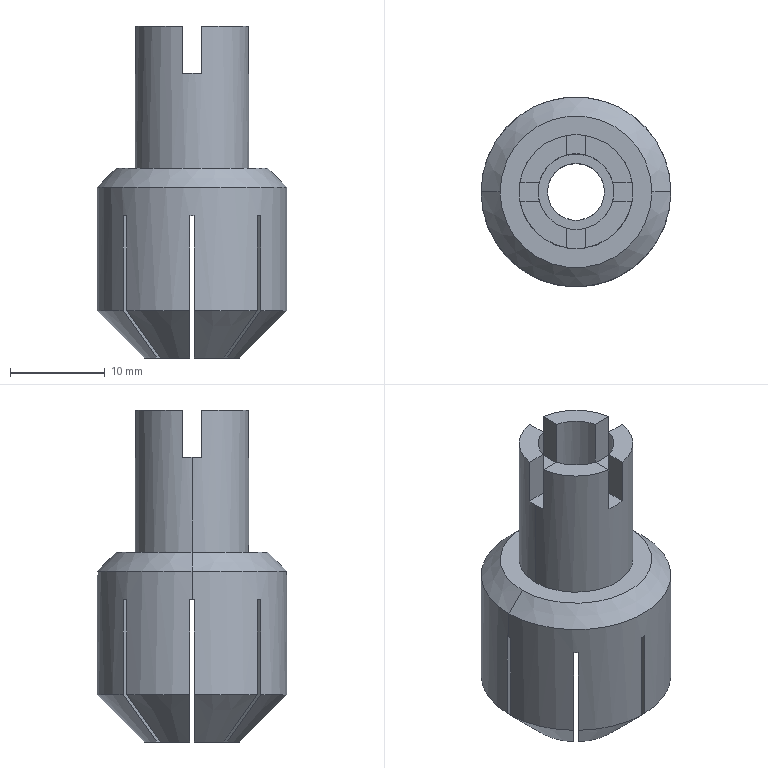Part | SolidWorks | features ICE 2, Chamfer 1, Revolution 1 | 1 solid | 68 faces | box 20 x 20 x 35 mm | volume 5438 mm3 | plane 50 | cone 10 | cylinder 8 | commonest cylinder face diameters 6 x2 8 x2 12 x2 20 x2